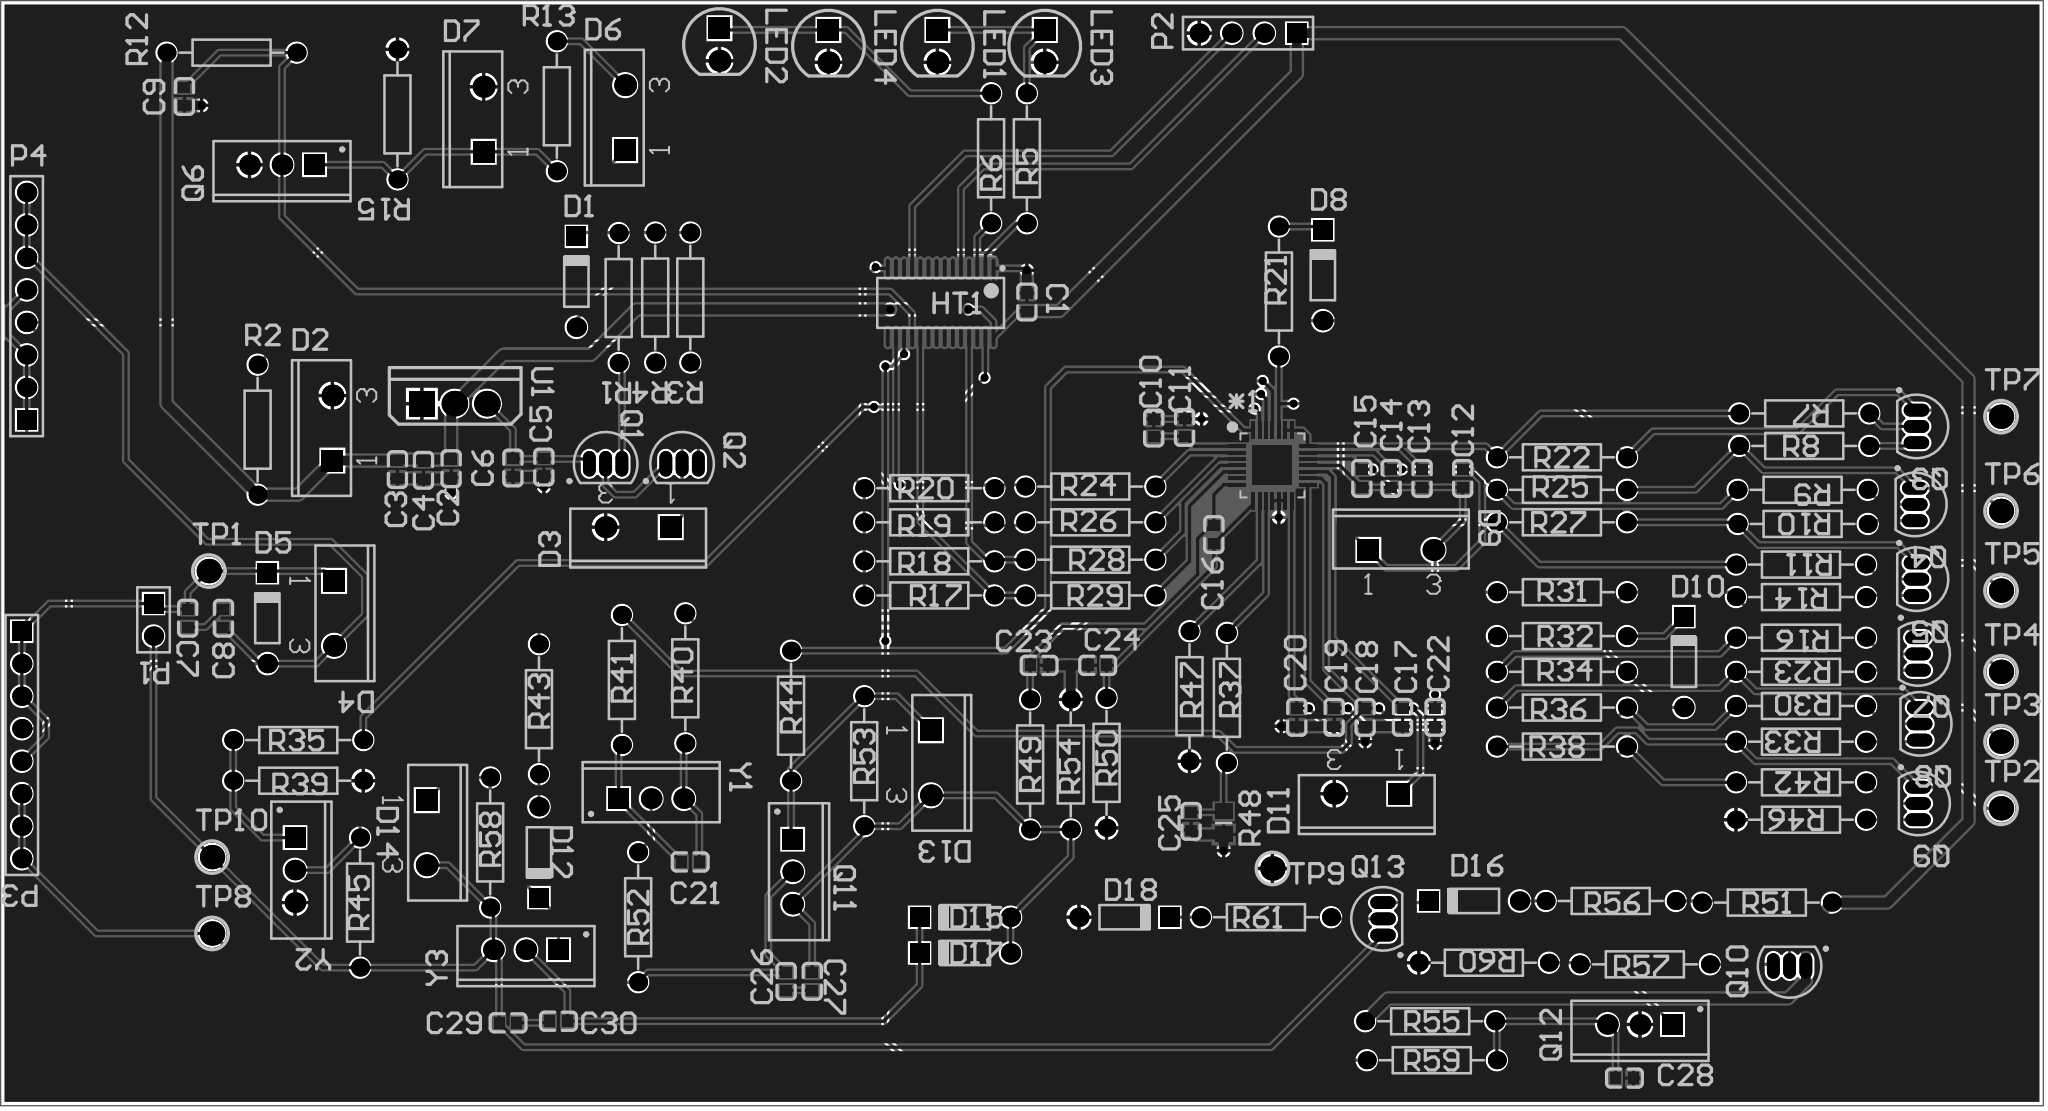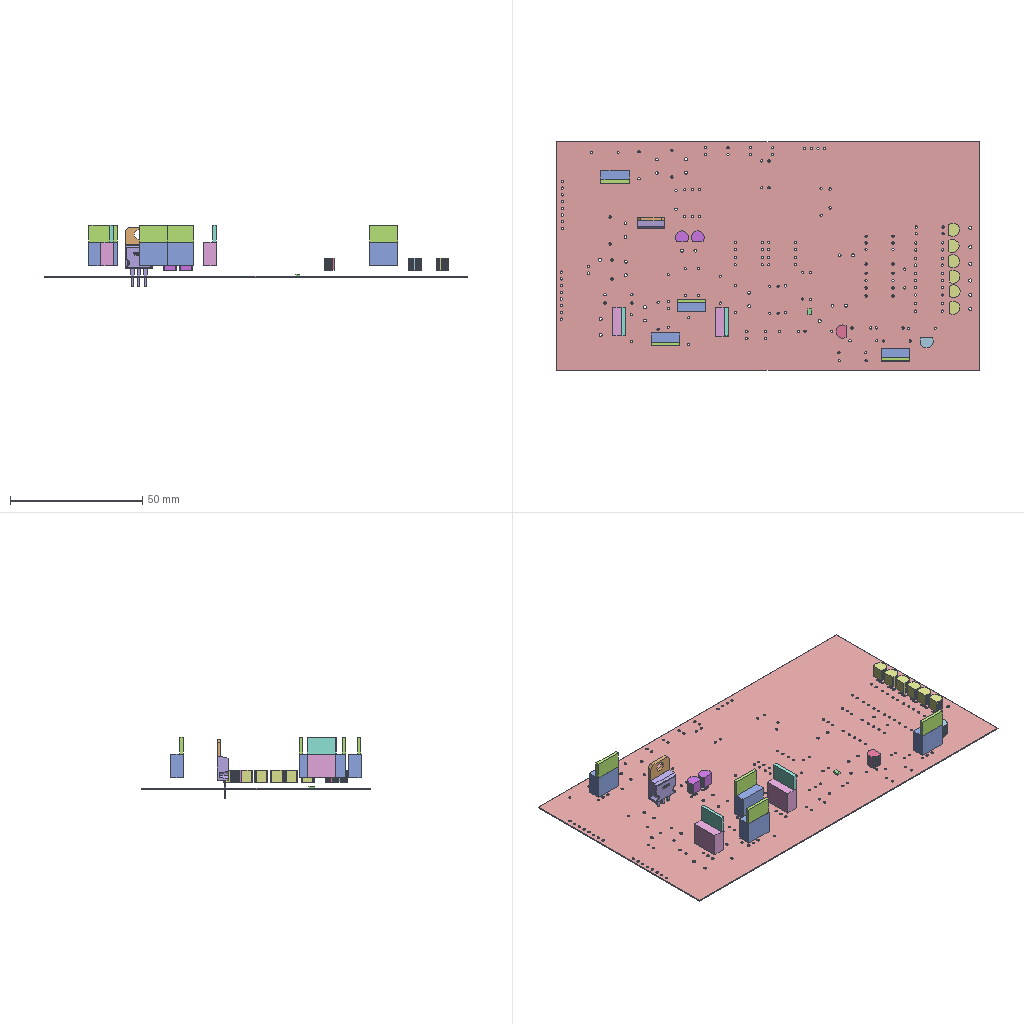Circuit board layout | Altium Designer | box 159.5 x 86.4 x 23.3 mm
Layer stack:
# Altium Designer layer stack of  (unit mm; dielectric type: 0 none, 1 core, 2 prepreg, 3 surface material)
index,name,kind,layer,copper_thickness_mm,dielectric_type,dielectric_thickness_mm,dielectric_material,dielectric_constant
0,Top Paste,other,,,,,,
1,Top Overlay,other,,,,,,
2,Top Solder,dielectric,,,3,0.0102,Solder Resist,3.5
3,Top Layer,copper,Top Layer,0.0356,,,,
4,Dielectric 1,dielectric,,,0,0.32,FR-4,4.8
5,Bottom Layer,copper,Bottom Layer,0.0356,,,,
6,Bottom Solder,dielectric,,,3,0.0102,Solder Resist,3.5
7,Bottom Overlay,other,,,,,,
8,Bottom Paste,other,,,,,,
# drill layer pairs: low layer,high layer
drill_pair,Top Layer,Bottom Layer
Part placement:
Designator,Comment,Layer,Footprint,Center-X(mm),Center-Y(mm),Rotation
Y3,NMOS-2,TopLayer,TO-220AB,66.421,37.592,180
Y2,NMOS-2,TopLayer,TO-220AB,48.387,43.815,270
Y1,NMOS-2,TopLayer,TO-220AB,76.2,49.403,360
U1,LM317,TopLayer,TO220A,60.833,80.264,360
TP10,TP-RED,TopLayer,TEST-TH_BD2.54-P1.4_RED,41.91,44.831,90
TP9,TP-RED,TopLayer,TEST-TH_BD2.54-P1.4_RED,124.714,43.942,0
TP8,TP-RED,TopLayer,TEST-TH_BD2.54-P1.4_RED,41.91,38.862,0
TP7,TP-RED,TopLayer,TEST-TH_BD2.54-P1.4_RED,181.61,79.248,0
TP6,TP-RED,TopLayer,TEST-TH_BD2.54-P1.4_RED,181.61,71.882,0
TP5,TP-RED,TopLayer,TEST-TH_BD2.54-P1.4_RED,181.61,65.659,0
TP4,TP-RED,TopLayer,TEST-TH_BD2.54-P1.4_RED,181.61,59.309,0
TP3,TP-RED,TopLayer,TEST-TH_BD2.54-P1.4_RED,181.61,53.848,0
TP2,TP-RED,TopLayer,TEST-TH_BD2.54-P1.4_RED,181.61,48.641,0
TP1,TP-RED,TopLayer,TEST-TH_BD2.54-P1.4_RED,41.656,67.183,0
R61,683,TopLayer,AXIAL-0.4,124.206,40.132,180
R60,105,TopLayer,AXIAL-0.4,141.224,36.576,180
R59,102,TopLayer,AXIAL-0.4,137.16,28.956,180
R58,104,TopLayer,AXIAL-0.4,63.627,45.974,90
R57,102,TopLayer,AXIAL-0.4,153.797,36.449,360
R56,104,TopLayer,AXIAL-0.4,151.13,41.402,360
R55,103,TopLayer,AXIAL-0.4,137.033,32.004,360
R54,101,TopLayer,AXIAL-0.4,108.966,52.07,270
R53,106,TopLayer,AXIAL-0.4,92.837,52.324,90
R52,104,TopLayer,AXIAL-0.4,75.184,40.132,90
R51,104,TopLayer,AXIAL-0.4,163.322,41.275,360
R50,101,TopLayer,AXIAL-0.4,111.76,52.197,90
R49,101,TopLayer,AXIAL-0.4,105.791,52.07,90
R48,Res Varistor,TopLayer,6-0805_N,120.904,47.498,90
R47,101,TopLayer,AXIAL-0.4,118.237,57.404,90
R46,68,TopLayer,AXIAL-0.4,165.989,47.752,180
R45,105,TopLayer,AXIAL-0.4,53.467,41.275,90
R44,102,TopLayer,AXIAL-0.4,87.122,55.88,90
R43,102,TopLayer,AXIAL-0.4,67.437,56.388,90
R42,511,TopLayer,AXIAL-0.4,165.989,50.673,360
R41,102,TopLayer,AXIAL-0.4,73.914,58.674,90
R40,102,TopLayer,AXIAL-0.4,78.867,58.801,90
R39,105,TopLayer,AXIAL-0.4,48.641,50.8,180
R38,102,TopLayer,AXIAL-0.4,147.32,53.467,180
R37,101,TopLayer,AXIAL-0.4,121.158,57.277,90
R36,102,TopLayer,AXIAL-0.4,147.32,56.515,180
R35,101,TopLayer,AXIAL-0.4,48.641,53.975,180
R34,102,TopLayer,AXIAL-0.4,147.32,59.309,360
R33,68,TopLayer,AXIAL-0.4,165.989,53.848,180
R32,51,TopLayer,AXIAL-0.4,147.32,62.103,360
R31,101,TopLayer,AXIAL-0.4,147.32,65.532,360
R30,511,TopLayer,AXIAL-0.4,165.989,56.642,360
R29,101,TopLayer,AXIAL-0.4,110.49,65.278,360
R28,101,TopLayer,AXIAL-0.4,110.49,68.072,360
R27,102,TopLayer,AXIAL-0.4,147.32,70.993,360
R26,101,TopLayer,AXIAL-0.4,110.49,70.993,360
R25,102,TopLayer,AXIAL-0.4,147.32,73.533,360
R24,101,TopLayer,AXIAL-0.4,110.49,73.787,360
R23,68,TopLayer,AXIAL-0.4,165.989,59.309,180
R22,102,TopLayer,AXIAL-0.4,147.32,76.073,360
R21,51,TopLayer,AXIAL-0.4,125.222,89.027,90
R20,103,TopLayer,AXIAL-0.4,97.917,73.66,180
R19,103,TopLayer,AXIAL-0.4,97.917,70.993,180
R18,103,TopLayer,AXIAL-0.4,97.917,67.945,180
R17,103,TopLayer,AXIAL-0.4,97.917,65.278,180
R16,511,TopLayer,AXIAL-0.4,165.989,61.976,360
R15,205,TopLayer,AXIAL-0.4,56.388,102.87,270
R14,68,TopLayer,AXIAL-0.4,165.989,65.151,180
R13,205,TopLayer,AXIAL-0.4,68.834,103.505,270
R12,105,TopLayer,AXIAL-0.4,43.434,107.696,180
R11,511,TopLayer,AXIAL-0.4,165.989,67.691,360
R10,68,TopLayer,AXIAL-0.4,166.116,70.866,180
R9,511,TopLayer,AXIAL-0.4,166.116,73.533,360
R8,68,TopLayer,AXIAL-0.4,166.243,76.962,180
R7,511,TopLayer,AXIAL-0.4,166.243,79.502,360
R6,621,TopLayer,AXIAL-0.4,102.743,99.441,270
R5,621,TopLayer,AXIAL-0.4,105.537,99.441,270
R4,475,TopLayer,AXIAL-0.4,76.516,88.559,270
R3,104,TopLayer,AXIAL-0.4,79.256,88.559,270
R2,NC,TopLayer,AXIAL-0.4,45.466,78.232,90
R1,10,TopLayer,AXIAL-0.4,73.66,88.519,270
Q13,2N3904,TopLayer,TO-92A,133.35,40.005,0
Q12,NMOS-2,TopLayer,TO-220AB,153.416,31.75,180
Q11,NMOS-2,TopLayer,TO-220AB,87.249,43.688,270
Q10,2N3906,TopLayer,TO-92A,165.1,36.322,90
Q9,2N3906,TopLayer,TO-92A,175.133,49.022,180
Q8,2N3906,TopLayer,TO-92A,175.26,55.245,180
Q7,2N3906,TopLayer,TO-92A,175.133,60.706,180
Q6,NMOS-2,TopLayer,TO-220AB,47.371,98.933,180
Q5,2N3906,TopLayer,TO-92A,175.006,66.548,180
Q4,2N3906,TopLayer,TO-92A,174.879,72.39,180
Q3,2N3906,TopLayer,TO-92A,175.006,78.486,180
Q2,2N3904,TopLayer,TO-92A,78.613,75.565,270
Q1,2N3904,TopLayer,TO-92A,72.644,75.565,270
P4,Header 8,TopLayer,HDR1X8,27.432,87.884,90
P3,Header 8,TopLayer,HDR1X8,27.051,53.594,270
P2,Header 4,TopLayer,HDR1X4,122.809,109.22,180
P1,Header 2,TopLayer,HDR1X2,37.338,63.373,270
LED4,I-LED,TopLayer,I-LED-5MM,90.043,108.204,270
LED3,I-LED,TopLayer,I-LED-5MM,106.934,108.204,270
LED2,I-LED,TopLayer,I-LED-5MM,81.534,108.331,270
LED1,I-LED,TopLayer,I-LED-5MM,98.552,108.204,270
HT1,HT66F3195,TopLayer,SSOP28_-_DUPLICATE,98.806,88.138,270
D18,1N4148,TopLayer,DO-35,113.157,40.132,360
D17,1N4148,TopLayer,DO-35,100.711,37.338,180
D16,1N4148,TopLayer,DO-35,140.462,41.402,180
D15,1N4148,TopLayer,DO-35,100.711,40.132,180
D14,MM3Z18,TopLayer,TO-220AC,58.674,46.736,270
D13,MM3Z18,TopLayer,TO-220AC,98.044,52.197,270
D12,1N4148,TopLayer,DO-35,67.437,45.212,270
D11,MM3Z18,TopLayer,TO-220AC,132.08,49.784,180
D10,Diode 1N4148,TopLayer,DO-35,156.845,60.071,90
D9,MM3Z18,TopLayer,TO-220AC,134.747,68.834,360
D8,Diode 1N4148,TopLayer,DO-35,128.651,90.297,90
D7,MM3Z18,TopLayer,TO-220AC,63.119,102.489,90
D6,MM3Z18,TopLayer,TO-220AC,74.168,102.616,90
D5,Diode 1N4148,TopLayer,DO-35,46.228,63.5,90
D4,MM3Z18,TopLayer,TO-220AC,51.435,63.881,270
D3,MM3Z18,TopLayer,TO-220AC,75.184,70.612,180
D2,MM3Z18,TopLayer,TO-220AC,51.308,78.359,90
D1,1N4148,TopLayer,DO-35,70.358,89.789,90
C30,104,TopLayer,C0603,68.953,32.007,180
C29,104,TopLayer,C0603,65.016,31.88,180
C28,103,TopLayer,C0603,152.211,27.559,360
C27,104,TopLayer,C0603,88.773,35.114,270
C26,104,TopLayer,C0603,86.741,35.117,90
C25,103,TopLayer,C0603,118.367,47.633,90
C24,104,TopLayer,C0603,111.06,59.817,180
C23,104,TopLayer,C0603,106.488,59.817,180
C22,225,TopLayer,C0603,137.417,55.761,90
C21,104,TopLayer,C0603,79.256,44.447,0
C20,104,TopLayer,C0603,126.619,55.761,90
C19,104,TopLayer,C0603,129.54,55.761,90
C18,104,TopLayer,C0603,131.956,55.761,90
C17,225,TopLayer,C0603,134.877,55.761,90
C16,104,TopLayer,C0603,120.142,70.042,90
C15,104,TopLayer,C0603,131.702,74.43,90
C14,104,TopLayer,C0603,133.988,74.43,90
C13,104,TopLayer,C0603,136.401,74.43,90
C12,225,TopLayer,C0603,139.576,74.43,90
C11,225,TopLayer,C0603,117.856,78.421,90
C10,104,TopLayer,C0603,115.446,78.367,90
C9,104,TopLayer,C0603,39.754,104.275,90
C8,104,TopLayer,C0603,42.802,63.508,90
C7,104,TopLayer,C0603,40.008,63.508,90
C6,104,TopLayer,C0603,65.405,75.246,90
C5,106,TopLayer,C0603,67.821,75.319,90
C4,104,TopLayer,C0603,58.423,75.065,90
C3,NC,TopLayer,C0603,56.388,75.122,90
C2,106,TopLayer,C0603,60.582,75.192,90
C1,104,TopLayer,C0603,105.537,88.2,270
*1,SH367306,TopLayer,QFN28L(5*5),124.714,75.438,0
Pad and via stacks:
# Altium Designer via and pad stacks of  (unit mm). Each distinct definition once, with the count of objects using it.
# via: kind,start_layer,end_layer,hole_mm,diameter_mm,mode(0 simple;1 top-mid-bottom;2 full stack),diameter_per_layer,count,example_net
# pad: kind,layer,hole_mm,hole_type(0 round;1 square;2 slot),plating,top_size,top_shape(1 round;2 rect;3 octagon;9 rounded rect),mid_size,bottom_size,mode,footprint,size_per_layer,count,example
pad,Top Layer,0,0,plated,0.25x1.4,2,0.25x1.4,0.25x1.4,0,QFN28L(5*5),,28,*1.28
pad,Top Layer,0,0,plated,3.1x3.1,2,3.1x3.1,3.1x3.1,0,QFN28L(5*5),,1,*1.29
pad,Top Layer,0,0,plated,0.8x0.9,2,0.8x0.9,0.8x0.9,0,C0603,,60,C30.1
pad,Top Layer,0,0,plated,0.3x1.5,1,0.3x1.5,0.3x1.5,0,SSOP28 - DUPLICATE,,28,HT1.1
pad,Top Layer,0,0,plated,1.4x1.2,2,1.4x1.2,1.4x1.2,0,6-0805_N,,2,R48.1
pad,Multi-Layer,1.1,0,plated,1.7x1.7,2,1.7x1.7,1.7x1.7,0,TO-220AC,,9,D14.1
pad,Multi-Layer,1.1,0,plated,1.7x1.7,1,1.7x1.7,1.7x1.7,0,TO-220AC,,9,D14.3
pad,Multi-Layer,0.9,0,plated,1.5x1.5,2,1.5x1.5,1.5x1.5,0,DO-35,,9,D18.2
pad,Multi-Layer,0.9,0,plated,1.5x1.5,1,1.5x1.5,1.5x1.5,0,DO-35,,9,D18.1
pad,Multi-Layer,0.9,0,plated,1.7x1.7,2,1.7x1.7,1.7x1.7,0,I-LED-5MM,,4,LED4.1
pad,Multi-Layer,0.9,0,plated,1.7x1.7,1,1.7x1.7,1.7x1.7,0,I-LED-5MM,,4,LED4.2
pad,Multi-Layer,0.9,0,plated,1.5x1.5,2,1.5x1.5,1.5x1.5,0,HDR1X2,,1,P1.1
pad,Multi-Layer,0.9,0,plated,1.5x1.5,1,1.5x1.5,1.5x1.5,0,HDR1X2,,1,P1.2
pad,Multi-Layer,0.9,0,plated,1.5x1.5,1,1.5x1.5,1.5x1.5,0,HDR1X4,,3,P2.4
pad,Multi-Layer,0.9,0,plated,1.5x1.5,2,1.5x1.5,1.5x1.5,0,HDR1X4,,1,P2.1
pad,Multi-Layer,0.9,0,plated,1.5x1.5,2,1.5x1.5,1.5x1.5,0,HDR1X8,,2,P4.1
pad,Multi-Layer,0.9,0,plated,1.5x1.5,1,1.5x1.5,1.5x1.5,0,HDR1X8,,14,P4.2
pad,Multi-Layer,0.9,0,plated,2x1,1,2x1,2x1,0,TO-92A,,30,Q13.3
pad,Multi-Layer,0.85,0,plated,1.4x1.4,1,1.4x1.4,1.4x1.4,0,AXIAL-0.4,,120,R61.1
pad,Multi-Layer,1.2,0,plated,1.9x1.9,1,1.9x1.9,1.9x1.9,0,TEST-TH_BD2.54-P1.4_RED,,10,TP10.1
pad,Multi-Layer,1.1,0,plated,2x2,1,2x2,2x2,0,TO220A,,2,U1.2
pad,Multi-Layer,1.1,0,plated,2x2,2,2x2,2x2,0,TO220A,,1,U1.1
pad,Multi-Layer,1,0,plated,1.6x1.6,1,1.6x1.6,1.6x1.6,0,TO-220AB,,12,Y3.3
pad,Multi-Layer,1,0,plated,1.6x1.6,2,1.6x1.6,1.6x1.6,0,TO-220AB,,6,Y3.1
via,Top Layer,Bottom Layer,0.3048,0.6096,0,,30,GND
Copper pours:
name,layer,net,type(0 solid;1 hatched;2 none)
G,Top Layer,GND,0
G,Bottom Layer,GND,0
Design rules, without the lines most boards share:
# Altium Designer design rules of  (exported by Altium Designer, unit mm)
# columns: name | kind | enabled | priority | scope1 | scope2 | descriptor | typed fields (field=value)
Clearance | 0 | enabled | 1 | All | All | Clearance Constraint (Gap=7mil) (All),(All) | gap=0.1778
PlaneConnect | 6 | enabled | 1 | All | All | Power Plane Connect Rule(Relief Connect )(Expansion=20mil) (Conductor Width=10mil) (Air Gap=10mil) (Entries=4) (All) | relief_conductor_width=0.254 relief_entries=4 relief_expansion=0.508
PolygonConnect | 20 | enabled | 1 | All | All | Polygon Connect Rule(Relief Connect )(Conductor Width=10mil) (Relief Angle=90 Angle) (Entries=4) (Air Gap Width=10mil) (All),(All) | connect_style(0=relief,1=direct,2=none)=0 relief_conductor_width=0.254 relief_entries=4
Width | 2 | enabled | 1 | All | All | Width Constraint (Min=10mil) (Max=30mil) (Preferred=10mil) (All) |
RoutingVias | 11 | enabled | 1 | All | All | Routing Via (MinHoleWidth=28mil) (MaxHoleWidth=28mil) (PreferredHoleWidth=28mil) (MinWidth=50mil) (MaxWidth=50mil) (PreferedWidth=50mil) (All) | via_min_hole=0.7112 via_max_hole=0.7112 via_preferred_diameter=1.27 via_preferred_hole=0.7112
SolderMaskExpansion | 13 | enabled | 1 | All | All | Solder Mask Expansion (Expansion =4mil) (All) | expansion=0.1016
DiffPairsRouting | 51 | enabled | 1 | All | All | Differential Pairs Uncoupled Length using the Gap Constraints (Min=10mil) (Max=10mil) (Prefered=10mil)  and Width Constraints (Min=15mil) (Max=15mil) (Prefered=15mil) (All) |
HoleToHoleClearance | 52 | enabled | 1 | All | All | Hole To Hole Clearance (Gap=10mil) (All),(All) | gap=0.254
MinimumSolderMaskSliver | 53 | enabled | 1 | All | All | Minimum Solder Mask Sliver (Gap=0mil) (All),(All) |
SilkToSolderMaskClearance | 54 | enabled | 1 | IsPad | All | Silk To Solder Mask (Clearance=0mil) (IsPad),(All) |
SilkToSilkClearance | 55 | enabled | 1 | All | All | Silk to Silk (Clearance=0mil) (All),(All) |
Classes set for this board:
# Altium Designer classes of  (member kind: 0 net, 1 component, 2 from-to, 3 pad, 4 layer, 5 differential pair, 6 design channel, 7 polygon, 8 structure, 9 xSignal)
# columns: class name | member kind | superclass | members
Sheet1 | 1 | no | *1; C1; C2; C3; C4; C5; C6; C7; C8; C9; C10; C11; C12; C13; C14; C15; C16; C17; C18; C19; C20; C21; C22; C23; C24; C25; C26; C27; C28; C29; C30; D1; D2; D3; D4; D5; D6; D7; D8; D9; D10; D11; D12; D13; D14; D15; D16; D17; D18; HT1; LED1; LED2; LED3; LED4; P1; P2; P3; P4; Q1; Q2; Q3; Q4; Q5; Q6; Q7; Q8; Q9; Q10; Q11; Q12; Q13; R1; R2; R3; R4; R5; R6; R7; R8; R9; R10; R11; R12; R13; R14; R15; R16; R17; R18; R19; R20; R21; R22; R23; R24; R25; R26; R27; R28; R29; R30; R31; R32; R33; R34; R35; R36; R37; R38; R39; R40; R41; R42; R43; R44; R45; R46; R47; R48; R49; R50; R51; R52; R53; R54; R55; R56; R57; R58; R59; R60; R61; TP1; TP2; TP3; TP4; TP5; TP6; TP7; TP8; TP9; TP10; U1; Y1; Y2; Y3;